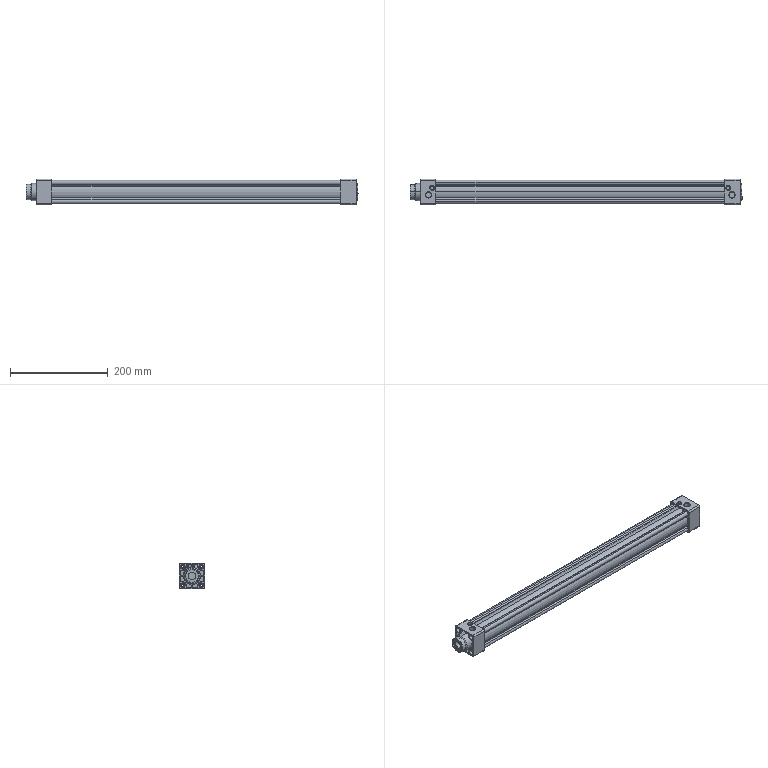Part | STEP file | SI_40x550-1 | 1 solid | 349 faces | box 679.5 x 53 x 53 mm | volume 489636 mm3 | cylinder 161 | plane 138 | cone 46 | spline 4 | commonest cylinder face diameters 8 x19 2 x18 6.5 x16 9.7 x16 4 x13 5.3 x8